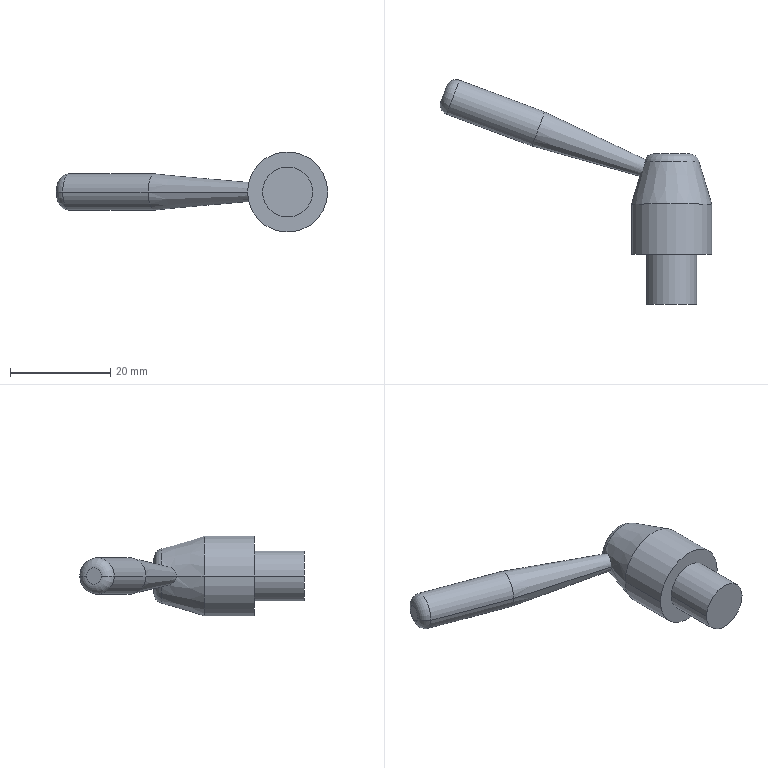Part | SolidWorks | features Revolution 2, Fillet 1, ICE 1 | 1 solid | 18 faces | box 54.148 x 44.825 x 16 mm | volume 5470 mm3 | cylinder 6 | cone 4 | plane 4 | torus 3 | spline 1 | commonest cylinder face diameters 7.237 x2 10 x2 16 x2
STEP:
#1=CARTESIAN_POINT('',(-46.023,30.491,0.));
#2=VERTEX_POINT('',#1);
#3=CARTESIAN_POINT('',(-44.892,33.524,0.));
#4=VERTEX_POINT('',#3);
#5=CARTESIAN_POINT('',(-45.457,32.007,0.));
#6=DIRECTION('',(-0.937,0.3493,0.));
#7=DIRECTION('',(0.3493,0.937,0.));
#8=AXIS2_PLACEMENT_3D('',#5,#6,#7);
#9=CIRCLE('',#8,1.618);
#10=EDGE_CURVE('',#2,#4,#9,.T.);
#11=ORIENTED_EDGE('',*,*,#10,.F.);
#12=CARTESIAN_POINT('',(-44.847,27.918,0.));
#13=VERTEX_POINT('',#12);
#14=CARTESIAN_POINT('',(-44.148,29.792,0.));
#15=DIRECTION('',(0.,0.,1.));
#16=DIRECTION('',(0.,-1.,0.));
#17=AXIS2_PLACEMENT_3D('',#14,#15,#16);
#18=CIRCLE('',#17,2.);
#19=EDGE_CURVE('',#2,#13,#18,.T.);
#20=ORIENTED_EDGE('',*,*,#19,.T.);
#21=CARTESIAN_POINT('',(-42.319,34.7,0.));
#22=VERTEX_POINT('',#21);
#23=CARTESIAN_POINT('',(-43.583,31.309,0.));
#24=DIRECTION('',(0.937,-0.3493,0.));
#25=DIRECTION('',(0.3493,0.937,0.));
#26=AXIS2_PLACEMENT_3D('',#23,#24,#25);
#27=CIRCLE('',#26,3.618);
#28=EDGE_CURVE('',#22,#13,#27,.T.);
#29=ORIENTED_EDGE('',*,*,#28,.F.);
#30=CARTESIAN_POINT('',(-43.018,32.825,0.));
#31=DIRECTION('',(0.,0.,-1.));
#32=DIRECTION('',(-1.,0.,0.));
#33=AXIS2_PLACEMENT_3D('',#30,#31,#32);
#34=CIRCLE('',#33,2.);
#35=EDGE_CURVE('',#4,#22,#34,.T.);
#36=ORIENTED_EDGE('',*,*,#35,.F.);
#37=EDGE_LOOP('',(#11,#20,#29,#36));
#38=FACE_OUTER_BOUND('',#37,.T.);
#39=CARTESIAN_POINT('',(-43.583,31.309,0.));
#40=DIRECTION('',(0.937,-0.3493,0.));
#41=DIRECTION('',(0.3493,0.937,0.));
#42=AXIS2_PLACEMENT_3D('',#39,#40,#41);
#43=TOROIDAL_SURFACE('',#42,1.618,2.);
#44=ADVANCED_FACE('',(#38),#43,.T.);
#45=CARTESIAN_POINT('',(5.,-10.,0.));
#46=VERTEX_POINT('',#45);
#47=CARTESIAN_POINT('',(-5.,-10.,0.));
#48=VERTEX_POINT('',#47);
#49=CARTESIAN_POINT('',(0.,-10.,0.));
#50=DIRECTION('',(0.,-1.,0.));
#51=DIRECTION('',(1.,0.,0.));
#52=AXIS2_PLACEMENT_3D('',#49,#50,#51);
#53=CIRCLE('',#52,5.);
#54=EDGE_CURVE('',#46,#48,#53,.T.);
#55=ORIENTED_EDGE('',*,*,#54,.F.);
#56=CARTESIAN_POINT('',(5.,0.,0.));
#57=VERTEX_POINT('',#56);
#58=CARTESIAN_POINT('',(5.,-10.,0.));
#59=DIRECTION('',(0.,1.,0.));
#60=VECTOR('',#59,1000.);
#61=LINE('',#58,#60);
#62=EDGE_CURVE('',#46,#57,#61,.T.);
#63=ORIENTED_EDGE('',*,*,#62,.T.);
#64=CARTESIAN_POINT('',(-5.,0.,0.));
#65=VERTEX_POINT('',#64);
#66=CARTESIAN_POINT('',(0.,0.,0.));
#67=DIRECTION('',(0.,-1.,0.));
#68=DIRECTION('',(1.,0.,0.));
#69=AXIS2_PLACEMENT_3D('',#66,#67,#68);
#70=CIRCLE('',#69,5.);
#71=EDGE_CURVE('',#57,#65,#70,.T.);
#72=ORIENTED_EDGE('',*,*,#71,.T.);
#73=CARTESIAN_POINT('',(-5.,-10.,0.));
#74=DIRECTION('',(0.,1.,0.));
#75=VECTOR('',#74,1000.);
#76=LINE('',#73,#75);
#77=EDGE_CURVE('',#48,#65,#76,.T.);
#78=ORIENTED_EDGE('',*,*,#77,.F.);
#79=EDGE_LOOP('',(#55,#63,#72,#78));
#80=FACE_OUTER_BOUND('',#79,.T.);
#81=CARTESIAN_POINT('',(0.,-10.,0.));
#82=DIRECTION('',(0.,1.,0.));
#83=DIRECTION('',(-1.,0.,0.));
#84=AXIS2_PLACEMENT_3D('',#81,#82,#83);
#85=CYLINDRICAL_SURFACE('',#84,5.);
#86=ADVANCED_FACE('',(#80),#85,.T.);
#87=CARTESIAN_POINT('',(-5.32,18.935,0.));
#88=VERTEX_POINT('',#87);
#89=CARTESIAN_POINT('',(-5.33,18.575,1.027));
#90=VERTEX_POINT('',#89);
#91=CARTESIAN_POINT('',(-5.32,18.935,0.));
#92=CARTESIAN_POINT('',(-5.32,18.935,0.184));
#93=CARTESIAN_POINT('',(-5.319,18.902,0.3697));
#94=CARTESIAN_POINT('',(-5.321,18.779,0.7171));
#95=CARTESIAN_POINT('',(-5.323,18.688,0.8817));
#96=CARTESIAN_POINT('',(-5.33,18.575,1.027));
#97=B_SPLINE_CURVE_WITH_KNOTS('',3,(#91,#92,#93,#94,#95,#96),.UNSPECIFIED.,.F.,.F.,(4,2,4),(0.003145,0.003696,0.004248),.UNSPECIFIED.);
#98=EDGE_CURVE('',#88,#90,#97,.T.);
#99=ORIENTED_EDGE('',*,*,#98,.F.);
#100=CARTESIAN_POINT('',(-25.317,28.362,0.));
#101=VERTEX_POINT('',#100);
#102=CARTESIAN_POINT('',(-25.317,28.362,0.));
#103=DIRECTION('',(-0.9045,0.4264,0.));
#104=VECTOR('',#103,1000.);
#105=LINE('',#102,#104);
#106=EDGE_CURVE('',#88,#101,#105,.T.);
#107=ORIENTED_EDGE('',*,*,#106,.T.);
#108=CARTESIAN_POINT('',(-27.844,21.581,0.));
#109=VERTEX_POINT('',#108);
#110=CARTESIAN_POINT('',(-26.581,24.972,0.));
#111=DIRECTION('',(0.937,-0.3493,0.));
#112=DIRECTION('',(0.3493,0.937,0.));
#113=AXIS2_PLACEMENT_3D('',#110,#111,#112);
#114=CIRCLE('',#113,3.618);
#115=EDGE_CURVE('',#101,#109,#114,.T.);
#116=ORIENTED_EDGE('',*,*,#115,.T.);
#117=CARTESIAN_POINT('',(-6.333,15.558,0.));
#118=VERTEX_POINT('',#117);
#119=CARTESIAN_POINT('',(-27.844,21.581,0.));
#120=DIRECTION('',(-0.963,0.2696,0.));
#121=VECTOR('',#120,1000.);
#122=LINE('',#119,#121);
#123=EDGE_CURVE('',#118,#109,#122,.T.);
#124=ORIENTED_EDGE('',*,*,#123,.F.);
#125=CARTESIAN_POINT('',(-5.33,18.575,1.027));
#126=CARTESIAN_POINT('',(-5.342,18.349,1.317));
#127=CARTESIAN_POINT('',(-5.375,18.033,1.538));
#128=CARTESIAN_POINT('',(-5.485,17.519,1.707));
#129=CARTESIAN_POINT('',(-5.531,17.342,1.737));
#130=CARTESIAN_POINT('',(-5.641,16.989,1.739));
#131=CARTESIAN_POINT('',(-5.704,16.818,1.712));
#132=CARTESIAN_POINT('',(-5.838,16.491,1.601));
#133=CARTESIAN_POINT('',(-5.907,16.341,1.519));
#134=CARTESIAN_POINT('',(-6.041,16.069,1.305));
#135=CARTESIAN_POINT('',(-6.104,15.953,1.177));
#136=CARTESIAN_POINT('',(-6.212,15.759,0.8805));
#137=CARTESIAN_POINT('',(-6.256,15.685,0.7177));
#138=CARTESIAN_POINT('',(-6.317,15.583,0.3675));
#139=CARTESIAN_POINT('',(-6.333,15.558,0.1844));
#140=CARTESIAN_POINT('',(-6.333,15.558,0.));
#141=B_SPLINE_CURVE_WITH_KNOTS('',3,(#125,#126,#127,#128,#129,#130,#131,#132,#133,#134,#135,#136,#137,#138,#139,#140),.UNSPECIFIED.,.F.,.F.,(4,2,2,2,2,2,2,4),(0.004248,0.005347,0.005897,0.006447,0.006996,0.007546,0.008096,0.008646),.UNSPECIFIED.);
#142=EDGE_CURVE('',#90,#118,#141,.T.);
#143=ORIENTED_EDGE('',*,*,#142,.F.);
#144=EDGE_LOOP('',(#99,#107,#116,#124,#143));
#145=FACE_OUTER_BOUND('',#144,.T.);
#146=CARTESIAN_POINT('',(-26.581,24.972,0.));
#147=DIRECTION('',(-0.937,0.3493,0.));
#148=DIRECTION('',(-0.3493,-0.937,0.));
#149=AXIS2_PLACEMENT_3D('',#146,#147,#148);
#150=CONICAL_SURFACE('',#149,3.618,0.08376);
#151=ADVANCED_FACE('',(#145),#150,.T.);
#152=ORIENTED_EDGE('',*,*,#28,.T.);
#153=CARTESIAN_POINT('',(-4.91,13.033,0.));
#154=DIRECTION('',(0.937,-0.3493,0.));
#155=VECTOR('',#154,1000.);
#156=LINE('',#153,#155);
#157=EDGE_CURVE('',#13,#109,#156,.T.);
#158=ORIENTED_EDGE('',*,*,#157,.T.);
#159=ORIENTED_EDGE('',*,*,#115,.F.);
#160=CARTESIAN_POINT('',(-2.383,19.814,0.));
#161=DIRECTION('',(0.937,-0.3493,0.));
#162=VECTOR('',#161,1000.);
#163=LINE('',#160,#162);
#164=EDGE_CURVE('',#22,#101,#163,.T.);
#165=ORIENTED_EDGE('',*,*,#164,.F.);
#166=EDGE_LOOP('',(#152,#158,#159,#165));
#167=FACE_OUTER_BOUND('',#166,.T.);
#168=CARTESIAN_POINT('',(-3.646,16.423,0.));
#169=DIRECTION('',(0.937,-0.3493,0.));
#170=DIRECTION('',(0.3493,0.937,0.));
#171=AXIS2_PLACEMENT_3D('',#168,#169,#170);
#172=CYLINDRICAL_SURFACE('',#171,3.618);
#173=ADVANCED_FACE('',(#167),#172,.T.);
#174=CARTESIAN_POINT('',(-8.,0.,0.));
#175=VERTEX_POINT('',#174);
#176=CARTESIAN_POINT('',(8.,0.,0.));
#177=VERTEX_POINT('',#176);
#178=CARTESIAN_POINT('',(0.,0.,0.));
#179=DIRECTION('',(0.,1.,0.));
#180=DIRECTION('',(-1.,0.,0.));
#181=AXIS2_PLACEMENT_3D('',#178,#179,#180);
#182=CIRCLE('',#181,8.);
#183=EDGE_CURVE('',#175,#177,#182,.T.);
#184=ORIENTED_EDGE('',*,*,#183,.T.);
#185=CARTESIAN_POINT('',(8.,10.,0.));
#186=VERTEX_POINT('',#185);
#187=CARTESIAN_POINT('',(8.,20.,0.));
#188=DIRECTION('',(0.,1.,0.));
#189=VECTOR('',#188,1000.);
#190=LINE('',#187,#189);
#191=EDGE_CURVE('',#177,#186,#190,.T.);
#192=ORIENTED_EDGE('',*,*,#191,.T.);
#193=CARTESIAN_POINT('',(-8.,10.,0.));
#194=VERTEX_POINT('',#193);
#195=CARTESIAN_POINT('',(0.,10.,0.));
#196=DIRECTION('',(0.,1.,0.));
#197=DIRECTION('',(-1.,0.,0.));
#198=AXIS2_PLACEMENT_3D('',#195,#196,#197);
#199=CIRCLE('',#198,8.);
#200=EDGE_CURVE('',#194,#186,#199,.T.);
#201=ORIENTED_EDGE('',*,*,#200,.F.);
#202=CARTESIAN_POINT('',(-8.,20.,0.));
#203=DIRECTION('',(0.,1.,0.));
#204=VECTOR('',#203,1000.);
#205=LINE('',#202,#204);
#206=EDGE_CURVE('',#175,#194,#205,.T.);
#207=ORIENTED_EDGE('',*,*,#206,.F.);
#208=EDGE_LOOP('',(#184,#192,#201,#207));
#209=FACE_OUTER_BOUND('',#208,.T.);
#210=CARTESIAN_POINT('',(0.,20.,0.));
#211=DIRECTION('',(0.,1.,0.));
#212=DIRECTION('',(-1.,0.,0.));
#213=AXIS2_PLACEMENT_3D('',#210,#211,#212);
#214=CYLINDRICAL_SURFACE('',#213,8.);
#215=ADVANCED_FACE('',(#209),#214,.T.);
#216=ORIENTED_EDGE('',*,*,#142,.T.);
#217=CARTESIAN_POINT('',(-5.,20.,0.));
#218=DIRECTION('',(-0.2873,-0.9578,0.));
#219=VECTOR('',#218,1000.);
#220=LINE('',#217,#219);
#221=EDGE_CURVE('',#118,#194,#220,.T.);
#222=ORIENTED_EDGE('',*,*,#221,.T.);
#223=ORIENTED_EDGE('',*,*,#200,.T.);
#224=CARTESIAN_POINT('',(5.428,18.575,0.));
#225=VERTEX_POINT('',#224);
#226=CARTESIAN_POINT('',(5.,20.,0.));
#227=DIRECTION('',(0.2873,-0.9578,0.));
#228=VECTOR('',#227,1000.);
#229=LINE('',#226,#228);
#230=EDGE_CURVE('',#225,#186,#229,.T.);
#231=ORIENTED_EDGE('',*,*,#230,.F.);
#232=CARTESIAN_POINT('',(0.,18.575,0.));
#233=DIRECTION('',(0.,-1.,0.));
#234=DIRECTION('',(-1.,0.,0.));
#235=AXIS2_PLACEMENT_3D('',#232,#233,#234);
#236=CIRCLE('',#235,5.428);
#237=EDGE_CURVE('',#225,#90,#236,.T.);
#238=ORIENTED_EDGE('',*,*,#237,.T.);
#239=EDGE_LOOP('',(#216,#222,#223,#231,#238));
#240=FACE_OUTER_BOUND('',#239,.T.);
#241=CARTESIAN_POINT('',(0.,20.,0.));
#242=DIRECTION('',(0.,-1.,0.));
#243=DIRECTION('',(1.,0.,0.));
#244=AXIS2_PLACEMENT_3D('',#241,#242,#243);
#245=CONICAL_SURFACE('',#244,5.,0.2915);
#246=ADVANCED_FACE('',(#240),#245,.T.);
#247=ORIENTED_EDGE('',*,*,#221,.F.);
#248=CARTESIAN_POINT('',(-5.33,18.575,-1.027));
#249=VERTEX_POINT('',#248);
#250=CARTESIAN_POINT('',(-6.333,15.558,0.));
#251=CARTESIAN_POINT('',(-6.333,15.558,-0.1843));
#252=CARTESIAN_POINT('',(-6.317,15.583,-0.3681));
#253=CARTESIAN_POINT('',(-6.256,15.684,-0.717));
#254=CARTESIAN_POINT('',(-6.212,15.76,-0.882));
#255=CARTESIAN_POINT('',(-6.05,16.049,-1.323));
#256=CARTESIAN_POINT('',(-5.904,16.33,-1.546));
#257=CARTESIAN_POINT('',(-5.704,16.817,-1.711));
#258=CARTESIAN_POINT('',(-5.641,16.991,-1.739));
#259=CARTESIAN_POINT('',(-5.531,17.342,-1.737));
#260=CARTESIAN_POINT('',(-5.485,17.521,-1.707));
#261=CARTESIAN_POINT('',(-5.412,17.862,-1.594));
#262=CARTESIAN_POINT('',(-5.385,18.028,-1.511));
#263=CARTESIAN_POINT('',(-5.347,18.326,-1.301));
#264=CARTESIAN_POINT('',(-5.336,18.463,-1.172));
#265=CARTESIAN_POINT('',(-5.33,18.575,-1.027));
#266=B_SPLINE_CURVE_WITH_KNOTS('',3,(#250,#251,#252,#253,#254,#255,#256,#257,#258,#259,#260,#261,#262,#263,#264,#265),.UNSPECIFIED.,.F.,.F.,(4,2,2,2,2,2,2,4),(0.008646,0.009195,0.009744,0.01084,0.01139,0.01194,0.01249,0.01304),.UNSPECIFIED.);
#267=EDGE_CURVE('',#118,#249,#266,.T.);
#268=ORIENTED_EDGE('',*,*,#267,.T.);
#269=CARTESIAN_POINT('',(0.,18.575,0.));
#270=DIRECTION('',(0.,-1.,0.));
#271=DIRECTION('',(-1.,0.,0.));
#272=AXIS2_PLACEMENT_3D('',#269,#270,#271);
#273=CIRCLE('',#272,5.428);
#274=EDGE_CURVE('',#249,#225,#273,.T.);
#275=ORIENTED_EDGE('',*,*,#274,.T.);
#276=ORIENTED_EDGE('',*,*,#230,.T.);
#277=CARTESIAN_POINT('',(0.,10.,0.));
#278=DIRECTION('',(0.,1.,0.));
#279=DIRECTION('',(-1.,0.,0.));
#280=AXIS2_PLACEMENT_3D('',#277,#278,#279);
#281=CIRCLE('',#280,8.);
#282=EDGE_CURVE('',#186,#194,#281,.T.);
#283=ORIENTED_EDGE('',*,*,#282,.T.);
#284=EDGE_LOOP('',(#247,#268,#275,#276,#283));
#285=FACE_OUTER_BOUND('',#284,.T.);
#286=CARTESIAN_POINT('',(0.,20.,0.));
#287=DIRECTION('',(0.,-1.,0.));
#288=DIRECTION('',(1.,0.,0.));
#289=AXIS2_PLACEMENT_3D('',#286,#287,#288);
#290=CONICAL_SURFACE('',#289,5.,0.2915);
#291=ADVANCED_FACE('',(#285),#290,.T.);
#292=CARTESIAN_POINT('',(0.,0.,0.));
#293=DIRECTION('',(0.,-1.,0.));
#294=DIRECTION('',(1.,0.,0.));
#295=AXIS2_PLACEMENT_3D('',#292,#293,#294);
#296=CIRCLE('',#295,5.);
#297=EDGE_CURVE('',#65,#57,#296,.T.);
#298=ORIENTED_EDGE('',*,*,#297,.F.);
#299=ORIENTED_EDGE('',*,*,#71,.F.);
#300=EDGE_LOOP('',(#298,#299));
#301=FACE_BOUND('',#300,.T.);
#302=ORIENTED_EDGE('',*,*,#183,.F.);
#303=CARTESIAN_POINT('',(0.,0.,0.));
#304=DIRECTION('',(0.,1.,0.));
#305=DIRECTION('',(-1.,0.,0.));
#306=AXIS2_PLACEMENT_3D('',#303,#304,#305);
#307=CIRCLE('',#306,8.);
#308=EDGE_CURVE('',#177,#175,#307,.T.);
#309=ORIENTED_EDGE('',*,*,#308,.F.);
#310=EDGE_LOOP('',(#302,#309));
#311=FACE_OUTER_BOUND('',#310,.T.);
#312=CARTESIAN_POINT('',(-8.,0.,0.));
#313=DIRECTION('',(0.,-1.,0.));
#314=DIRECTION('',(1.,0.,0.));
#315=AXIS2_PLACEMENT_3D('',#312,#313,#314);
#316=PLANE('',#315);
#317=ADVANCED_FACE('',(#301,#311),#316,.T.);
#318=CARTESIAN_POINT('',(-3.448,20.,0.6647));
#319=VERTEX_POINT('',#318);
#320=CARTESIAN_POINT('',(-3.448,20.,-0.6647));
#321=VERTEX_POINT('',#320);
#322=CARTESIAN_POINT('',(0.,20.,0.));
#323=DIRECTION('',(0.,1.,0.));
#324=DIRECTION('',(-1.,0.,0.));
#325=AXIS2_PLACEMENT_3D('',#322,#323,#324);
#326=CIRCLE('',#325,3.512);
#327=EDGE_CURVE('',#319,#321,#326,.T.);
#328=ORIENTED_EDGE('',*,*,#327,.T.);
#329=CARTESIAN_POINT('',(-3.448,20.,-0.6647));
#330=CARTESIAN_POINT('',(-3.47,20.,-0.5552));
#331=CARTESIAN_POINT('',(-3.494,20.,-0.4458));
#332=CARTESIAN_POINT('',(-3.535,20.,-0.2268));
#333=CARTESIAN_POINT('',(-3.551,20.,-0.117));
#334=CARTESIAN_POINT('',(-3.552,20.,0.1047));
#335=CARTESIAN_POINT('',(-3.536,20.,0.2166));
#336=CARTESIAN_POINT('',(-3.495,20.,0.4409));
#337=CARTESIAN_POINT('',(-3.47,20.,0.5525));
#338=CARTESIAN_POINT('',(-3.448,20.,0.6647));
#339=B_SPLINE_CURVE_WITH_KNOTS('',3,(#329,#330,#331,#332,#333,#334,#335,#336,#337,#338),.UNSPECIFIED.,.F.,.F.,(4,2,2,2,4),(0.,0.0003319,0.0006638,0.0009957,0.001328),.UNSPECIFIED.);
#340=EDGE_CURVE('',#321,#319,#339,.T.);
#341=ORIENTED_EDGE('',*,*,#340,.T.);
#342=EDGE_LOOP('',(#328,#341));
#343=FACE_OUTER_BOUND('',#342,.T.);
#344=CARTESIAN_POINT('',(-5.,20.,0.));
#345=DIRECTION('',(0.,1.,0.));
#346=DIRECTION('',(-1.,0.,0.));
#347=AXIS2_PLACEMENT_3D('',#344,#345,#346);
#348=PLANE('',#347);
#349=ADVANCED_FACE('',(#343),#348,.T.);
#350=ORIENTED_EDGE('',*,*,#191,.F.);
#351=ORIENTED_EDGE('',*,*,#308,.T.);
#352=ORIENTED_EDGE('',*,*,#206,.T.);
#353=ORIENTED_EDGE('',*,*,#282,.F.);
#354=EDGE_LOOP('',(#350,#351,#352,#353));
#355=FACE_OUTER_BOUND('',#354,.T.);
#356=CARTESIAN_POINT('',(0.,20.,0.));
#357=DIRECTION('',(0.,1.,0.));
#358=DIRECTION('',(-1.,0.,0.));
#359=AXIS2_PLACEMENT_3D('',#356,#357,#358);
#360=CYLINDRICAL_SURFACE('',#359,8.);
#361=ADVANCED_FACE('',(#355),#360,.T.);
#362=CARTESIAN_POINT('',(-45.457,32.007,0.));
#363=DIRECTION('',(-0.937,0.3493,0.));
#364=DIRECTION('',(0.3493,0.937,0.));
#365=AXIS2_PLACEMENT_3D('',#362,#363,#364);
#366=CIRCLE('',#365,1.618);
#367=EDGE_CURVE('',#4,#2,#366,.T.);
#368=ORIENTED_EDGE('',*,*,#367,.T.);
#369=ORIENTED_EDGE('',*,*,#10,.T.);
#370=EDGE_LOOP('',(#368,#369));
#371=FACE_OUTER_BOUND('',#370,.T.);
#372=CARTESIAN_POINT('',(-45.457,32.007,0.));
#373=DIRECTION('',(0.937,-0.3493,0.));
#374=DIRECTION('',(0.3493,0.937,0.));
#375=AXIS2_PLACEMENT_3D('',#372,#373,#374);
#376=PLANE('',#375);
#377=ADVANCED_FACE('',(#371),#376,.F.);
#378=ORIENTED_EDGE('',*,*,#157,.F.);
#379=CARTESIAN_POINT('',(-43.583,31.309,0.));
#380=DIRECTION('',(0.937,-0.3493,0.));
#381=DIRECTION('',(0.3493,0.937,0.));
#382=AXIS2_PLACEMENT_3D('',#379,#380,#381);
#383=CIRCLE('',#382,3.618);
#384=EDGE_CURVE('',#13,#22,#383,.T.);
#385=ORIENTED_EDGE('',*,*,#384,.T.);
#386=ORIENTED_EDGE('',*,*,#164,.T.);
#387=CARTESIAN_POINT('',(-26.581,24.972,0.));
#388=DIRECTION('',(0.937,-0.3493,0.));
#389=DIRECTION('',(0.3493,0.937,0.));
#390=AXIS2_PLACEMENT_3D('',#387,#388,#389);
#391=CIRCLE('',#390,3.618);
#392=EDGE_CURVE('',#109,#101,#391,.T.);
#393=ORIENTED_EDGE('',*,*,#392,.F.);
#394=EDGE_LOOP('',(#378,#385,#386,#393));
#395=FACE_OUTER_BOUND('',#394,.T.);
#396=CARTESIAN_POINT('',(-3.646,16.423,0.));
#397=DIRECTION('',(0.937,-0.3493,0.));
#398=DIRECTION('',(0.3493,0.937,0.));
#399=AXIS2_PLACEMENT_3D('',#396,#397,#398);
#400=CYLINDRICAL_SURFACE('',#399,3.618);
#401=ADVANCED_FACE('',(#395),#400,.T.);
#402=ORIENTED_EDGE('',*,*,#106,.F.);
#403=CARTESIAN_POINT('',(-5.33,18.575,-1.027));
#404=CARTESIAN_POINT('',(-5.323,18.687,-0.8821));
#405=CARTESIAN_POINT('',(-5.321,18.779,-0.7167));
#406=CARTESIAN_POINT('',(-5.319,18.902,-0.3703));
#407=CARTESIAN_POINT('',(-5.32,18.935,-0.1842));
#408=CARTESIAN_POINT('',(-5.32,18.935,0.));
#409=B_SPLINE_CURVE_WITH_KNOTS('',3,(#403,#404,#405,#406,#407,#408),.UNSPECIFIED.,.F.,.F.,(4,2,4),(0.002041,0.002593,0.003145),.UNSPECIFIED.);
#410=EDGE_CURVE('',#249,#88,#409,.T.);
#411=ORIENTED_EDGE('',*,*,#410,.F.);
#412=ORIENTED_EDGE('',*,*,#267,.F.);
#413=ORIENTED_EDGE('',*,*,#123,.T.);
#414=ORIENTED_EDGE('',*,*,#392,.T.);
#415=EDGE_LOOP('',(#402,#411,#412,#413,#414));
#416=FACE_OUTER_BOUND('',#415,.T.);
#417=CARTESIAN_POINT('',(-26.581,24.972,0.));
#418=DIRECTION('',(-0.937,0.3493,0.));
#419=DIRECTION('',(-0.3493,-0.937,0.));
#420=AXIS2_PLACEMENT_3D('',#417,#418,#419);
#421=CONICAL_SURFACE('',#420,3.618,0.08376);
#422=ADVANCED_FACE('',(#416),#421,.T.);
#423=ORIENTED_EDGE('',*,*,#62,.F.);
#424=CARTESIAN_POINT('',(0.,-10.,0.));
#425=DIRECTION('',(0.,-1.,0.));
#426=DIRECTION('',(1.,0.,0.));
#427=AXIS2_PLACEMENT_3D('',#424,#425,#426);
#428=CIRCLE('',#427,5.);
#429=EDGE_CURVE('',#48,#46,#428,.T.);
#430=ORIENTED_EDGE('',*,*,#429,.F.);
#431=ORIENTED_EDGE('',*,*,#77,.T.);
#432=ORIENTED_EDGE('',*,*,#297,.T.);
#433=EDGE_LOOP('',(#423,#430,#431,#432));
#434=FACE_OUTER_BOUND('',#433,.T.);
#435=CARTESIAN_POINT('',(0.,-10.,0.));
#436=DIRECTION('',(0.,1.,0.));
#437=DIRECTION('',(-1.,0.,0.));
#438=AXIS2_PLACEMENT_3D('',#435,#436,#437);
#439=CYLINDRICAL_SURFACE('',#438,5.);
#440=ADVANCED_FACE('',(#434),#439,.T.);
#441=ORIENTED_EDGE('',*,*,#429,.T.);
#442=ORIENTED_EDGE('',*,*,#54,.T.);
#443=EDGE_LOOP('',(#441,#442));
#444=FACE_OUTER_BOUND('',#443,.T.);
#445=CARTESIAN_POINT('',(0.,-10.,0.));
#446=DIRECTION('',(0.,-1.,0.));
#447=DIRECTION('',(1.,0.,0.));
#448=AXIS2_PLACEMENT_3D('',#445,#446,#447);
#449=PLANE('',#448);
#450=ADVANCED_FACE('',(#444),#449,.T.);
#451=CARTESIAN_POINT('',(-3.448,18.,0.6647));
#452=DIRECTION('',(-0.1893,0.,-0.9819));
#453=DIRECTION('',(-0.9819,0.,0.1893));
#454=AXIS2_PLACEMENT_3D('',#451,#452,#453);
#455=CIRCLE('',#454,2.);
#456=EDGE_CURVE('',#90,#319,#455,.T.);
#457=ORIENTED_EDGE('',*,*,#456,.F.);
#458=ORIENTED_EDGE('',*,*,#237,.F.);
#459=ORIENTED_EDGE('',*,*,#274,.F.);
#460=CARTESIAN_POINT('',(-3.448,18.,-0.6647));
#461=DIRECTION('',(-0.1893,0.,0.9819));
#462=DIRECTION('',(0.9819,0.,0.1893));
#463=AXIS2_PLACEMENT_3D('',#460,#461,#462);
#464=CIRCLE('',#463,2.);
#465=EDGE_CURVE('',#321,#249,#464,.T.);
#466=ORIENTED_EDGE('',*,*,#465,.F.);
#467=ORIENTED_EDGE('',*,*,#327,.F.);
#468=EDGE_LOOP('',(#457,#458,#459,#466,#467));
#469=FACE_OUTER_BOUND('',#468,.T.);
#470=CARTESIAN_POINT('',(0.,18.,0.));
#471=DIRECTION('',(0.,1.,0.));
#472=DIRECTION('',(-1.,0.,0.));
#473=AXIS2_PLACEMENT_3D('',#470,#471,#472);
#474=TOROIDAL_SURFACE('',#473,3.512,2.);
#475=ADVANCED_FACE('',(#469),#474,.T.);
#476=ORIENTED_EDGE('',*,*,#465,.T.);
#477=ORIENTED_EDGE('',*,*,#410,.T.);
#478=ORIENTED_EDGE('',*,*,#98,.T.);
#479=ORIENTED_EDGE('',*,*,#456,.T.);
#480=ORIENTED_EDGE('',*,*,#340,.F.);
#481=EDGE_LOOP('',(#476,#477,#478,#479,#480));
#482=FACE_OUTER_BOUND('',#481,.T.);
#483=CARTESIAN_POINT('',(-3.448,20.,0.6647));
#484=CARTESIAN_POINT('',(-4.91,20.,0.9463));
#485=CARTESIAN_POINT('',(-5.33,18.575,1.027));
#486=CARTESIAN_POINT('',(-3.47,20.,0.554));
#487=CARTESIAN_POINT('',(-4.874,20.,0.8482));
#488=CARTESIAN_POINT('',(-5.326,18.642,0.9408));
#489=CARTESIAN_POINT('',(-3.494,20.,0.4433));
#490=CARTESIAN_POINT('',(-4.839,20.,0.7302));
#491=CARTESIAN_POINT('',(-5.323,18.717,0.8319));
#492=CARTESIAN_POINT('',(-3.525,20.,0.2772));
#493=CARTESIAN_POINT('',(-4.795,20.,0.4971));
#494=CARTESIAN_POINT('',(-5.32,18.827,0.5876));
#495=CARTESIAN_POINT('',(-3.534,20.,0.2219));
#496=CARTESIAN_POINT('',(-4.782,20.,0.4105));
#497=CARTESIAN_POINT('',(-5.32,18.862,0.4917));
#498=CARTESIAN_POINT('',(-3.548,20.,0.1112));
#499=CARTESIAN_POINT('',(-4.762,20.,0.2171));
#500=CARTESIAN_POINT('',(-5.32,18.917,0.2656));
#501=CARTESIAN_POINT('',(-3.551,20.,0.05579));
#502=CARTESIAN_POINT('',(-4.756,20.,0.1093));
#503=CARTESIAN_POINT('',(-5.32,18.935,0.1342));
#504=CARTESIAN_POINT('',(-3.551,20.,-0.05498));
#505=CARTESIAN_POINT('',(-4.756,20.,-0.1077));
#506=CARTESIAN_POINT('',(-5.32,18.935,-0.1323));
#507=CARTESIAN_POINT('',(-3.548,20.,-0.1104));
#508=CARTESIAN_POINT('',(-4.762,20.,-0.2157));
#509=CARTESIAN_POINT('',(-5.32,18.917,-0.2639));
#510=CARTESIAN_POINT('',(-3.535,20.,-0.2212));
#511=CARTESIAN_POINT('',(-4.782,20.,-0.4094));
#512=CARTESIAN_POINT('',(-5.32,18.863,-0.4905));
#513=CARTESIAN_POINT('',(-3.525,20.,-0.2766));
#514=CARTESIAN_POINT('',(-4.795,20.,-0.4962));
#515=CARTESIAN_POINT('',(-5.32,18.827,-0.5867));
#516=CARTESIAN_POINT('',(-3.494,20.,-0.4429));
#517=CARTESIAN_POINT('',(-4.839,20.,-0.7298));
#518=CARTESIAN_POINT('',(-5.323,18.718,-0.8316));
#519=CARTESIAN_POINT('',(-3.47,20.,-0.5538));
#520=CARTESIAN_POINT('',(-4.874,20.,-0.848));
#521=CARTESIAN_POINT('',(-5.326,18.642,-0.9406));
#522=CARTESIAN_POINT('',(-3.448,20.,-0.6647));
#523=CARTESIAN_POINT('',(-4.91,20.,-0.9463));
#524=CARTESIAN_POINT('',(-5.33,18.575,-1.027));
#525=(BOUNDED_SURFACE()B_SPLINE_SURFACE(3,2,((#483,#484,#485),(#486,#487,#488),(#489,#490,#491),(#492,#493,#494),(#495,#496,#497),(#498,#499,#500),(#501,#502,#503),(#504,#505,#506),(#507,#508,#509),(#510,#511,#512),(#513,#514,#515),(#516,#517,#518),(#519,#520,#521),(#522,#523,#524)),.UNSPECIFIED.,.F.,.F.,.T.)B_SPLINE_SURFACE_WITH_KNOTS((4,2,2,2,2,2,4),(3,3),(0.006156,0.006491,0.006658,0.006826,0.006993,0.00716,0.007495),(0.,1.),.UNSPECIFIED.)GEOMETRIC_REPRESENTATION_ITEM()RATIONAL_B_SPLINE_SURFACE(((1.,0.8023,1.),(1.,0.8126,1.),(1.,0.8243,1.),(1.,0.8407,1.),(1.,0.8459,1.),(1.,0.8539,1.),(1.,0.8565,1.),(1.,0.8566,1.),(1.,0.854,1.),(1.,0.846,1.),(1.,0.8407,1.),(1.,0.8243,1.),(1.,0.8126,1.),(1.,0.8023,1.)))REPRESENTATION_ITEM('')SURFACE());
#526=ADVANCED_FACE('',(#482),#525,.T.);
#527=ORIENTED_EDGE('',*,*,#19,.F.);
#528=ORIENTED_EDGE('',*,*,#367,.F.);
#529=ORIENTED_EDGE('',*,*,#35,.T.);
#530=ORIENTED_EDGE('',*,*,#384,.F.);
#531=EDGE_LOOP('',(#527,#528,#529,#530));
#532=FACE_OUTER_BOUND('',#531,.T.);
#533=CARTESIAN_POINT('',(-43.583,31.309,0.));
#534=DIRECTION('',(0.937,-0.3493,0.));
#535=DIRECTION('',(0.3493,0.937,0.));
#536=AXIS2_PLACEMENT_3D('',#533,#534,#535);
#537=TOROIDAL_SURFACE('',#536,1.618,2.);
#538=ADVANCED_FACE('',(#532),#537,.T.);
#539=CLOSED_SHELL('',(#44,#86,#151,#173,#215,#246,#291,#317,#349,#361,#377,#401,#422,#440,#450,#475,#526,#538));
#540=MANIFOLD_SOLID_BREP('',#539);
#541=CARTESIAN_POINT('',(0.,0.,0.));
#542=DIRECTION('',(0.,0.,1.));
#543=DIRECTION('',(1.,0.,0.));
#544=AXIS2_PLACEMENT_3D('',#541,#542,#543);
#545=(LENGTH_UNIT()NAMED_UNIT(*)SI_UNIT(.MILLI.,.METRE.));
#546=UNCERTAINTY_MEASURE_WITH_UNIT(LENGTH_MEASURE(0.00001),#545,'','');
#547=(NAMED_UNIT(*)PLANE_ANGLE_UNIT()SI_UNIT($,.RADIAN.));
#548=(NAMED_UNIT(*)SI_UNIT($,.STERADIAN.)SOLID_ANGLE_UNIT());
#549=(GEOMETRIC_REPRESENTATION_CONTEXT(3)GLOBAL_UNCERTAINTY_ASSIGNED_CONTEXT((#546))GLOBAL_UNIT_ASSIGNED_CONTEXT((#545,#547,#548))REPRESENTATION_CONTEXT('',''));
#550=ADVANCED_BREP_SHAPE_REPRESENTATION('',(#540,#544),#549);